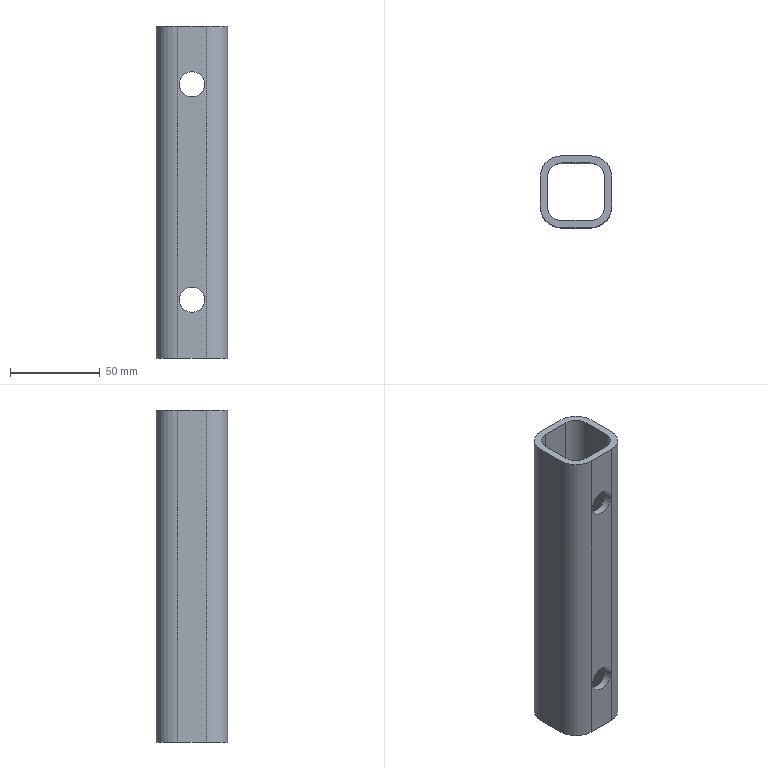Part | SolidWorks | features LayoutProfileFeature 1 | 1 solid | 26 faces | box 40 x 40 x 185 mm | volume 91393 mm3 | cylinder 16 | plane 10 | commonest cylinder face diameters 14 x8 16 x4 24 x4
STEP:
#1=CARTESIAN_POINT('',(7.,-20.,32.5));
#2=VERTEX_POINT('',#1);
#3=CARTESIAN_POINT('',(-7.,-20.,32.5));
#4=VERTEX_POINT('',#3);
#5=CARTESIAN_POINT('',(0.,-20.,32.5));
#6=DIRECTION('',(0.,1.,0.));
#7=DIRECTION('',(-1.,0.,0.));
#8=AXIS2_PLACEMENT_3D('',#5,#6,#7);
#9=CIRCLE('',#8,7.);
#10=EDGE_CURVE('',#2,#4,#9,.T.);
#11=ORIENTED_EDGE('',*,*,#10,.F.);
#12=CARTESIAN_POINT('',(7.,-16.,32.5));
#13=VERTEX_POINT('',#12);
#14=CARTESIAN_POINT('',(7.,-20.,32.5));
#15=DIRECTION('',(0.,1.,0.));
#16=VECTOR('',#15,1000.);
#17=LINE('',#14,#16);
#18=EDGE_CURVE('',#2,#13,#17,.T.);
#19=ORIENTED_EDGE('',*,*,#18,.T.);
#20=CARTESIAN_POINT('',(-7.,-16.,32.5));
#21=VERTEX_POINT('',#20);
#22=CARTESIAN_POINT('',(0.,-16.,32.5));
#23=DIRECTION('',(0.,1.,0.));
#24=DIRECTION('',(-1.,0.,0.));
#25=AXIS2_PLACEMENT_3D('',#22,#23,#24);
#26=CIRCLE('',#25,7.);
#27=EDGE_CURVE('',#13,#21,#26,.T.);
#28=ORIENTED_EDGE('',*,*,#27,.T.);
#29=CARTESIAN_POINT('',(-7.,-20.,32.5));
#30=DIRECTION('',(0.,1.,0.));
#31=VECTOR('',#30,1000.);
#32=LINE('',#29,#31);
#33=EDGE_CURVE('',#4,#21,#32,.T.);
#34=ORIENTED_EDGE('',*,*,#33,.F.);
#35=EDGE_LOOP('',(#11,#19,#28,#34));
#36=FACE_OUTER_BOUND('',#35,.T.);
#37=CARTESIAN_POINT('',(0.,-20.,32.5));
#38=DIRECTION('',(0.,1.,0.));
#39=DIRECTION('',(-1.,0.,0.));
#40=AXIS2_PLACEMENT_3D('',#37,#38,#39);
#41=CYLINDRICAL_SURFACE('',#40,7.);
#42=ADVANCED_FACE('',(#36),#41,.F.);
#43=CARTESIAN_POINT('',(7.,-20.,152.5));
#44=VERTEX_POINT('',#43);
#45=CARTESIAN_POINT('',(-7.,-20.,152.5));
#46=VERTEX_POINT('',#45);
#47=CARTESIAN_POINT('',(0.,-20.,152.5));
#48=DIRECTION('',(0.,1.,0.));
#49=DIRECTION('',(-1.,0.,0.));
#50=AXIS2_PLACEMENT_3D('',#47,#48,#49);
#51=CIRCLE('',#50,7.);
#52=EDGE_CURVE('',#44,#46,#51,.T.);
#53=ORIENTED_EDGE('',*,*,#52,.F.);
#54=CARTESIAN_POINT('',(7.,-16.,152.5));
#55=VERTEX_POINT('',#54);
#56=CARTESIAN_POINT('',(7.,-20.,152.5));
#57=DIRECTION('',(0.,1.,0.));
#58=VECTOR('',#57,1000.);
#59=LINE('',#56,#58);
#60=EDGE_CURVE('',#44,#55,#59,.T.);
#61=ORIENTED_EDGE('',*,*,#60,.T.);
#62=CARTESIAN_POINT('',(-7.,-16.,152.5));
#63=VERTEX_POINT('',#62);
#64=CARTESIAN_POINT('',(0.,-16.,152.5));
#65=DIRECTION('',(0.,1.,0.));
#66=DIRECTION('',(-1.,0.,0.));
#67=AXIS2_PLACEMENT_3D('',#64,#65,#66);
#68=CIRCLE('',#67,7.);
#69=EDGE_CURVE('',#55,#63,#68,.T.);
#70=ORIENTED_EDGE('',*,*,#69,.T.);
#71=CARTESIAN_POINT('',(-7.,-20.,152.5));
#72=DIRECTION('',(0.,1.,0.));
#73=VECTOR('',#72,1000.);
#74=LINE('',#71,#73);
#75=EDGE_CURVE('',#46,#63,#74,.T.);
#76=ORIENTED_EDGE('',*,*,#75,.F.);
#77=EDGE_LOOP('',(#53,#61,#70,#76));
#78=FACE_OUTER_BOUND('',#77,.T.);
#79=CARTESIAN_POINT('',(0.,-20.,152.5));
#80=DIRECTION('',(0.,1.,0.));
#81=DIRECTION('',(-1.,0.,0.));
#82=AXIS2_PLACEMENT_3D('',#79,#80,#81);
#83=CYLINDRICAL_SURFACE('',#82,7.);
#84=ADVANCED_FACE('',(#78),#83,.F.);
#85=CARTESIAN_POINT('',(-7.,16.,32.5));
#86=VERTEX_POINT('',#85);
#87=CARTESIAN_POINT('',(7.,16.,32.5));
#88=VERTEX_POINT('',#87);
#89=CARTESIAN_POINT('',(0.,16.,32.5));
#90=DIRECTION('',(0.,-1.,0.));
#91=DIRECTION('',(-1.,0.,0.));
#92=AXIS2_PLACEMENT_3D('',#89,#90,#91);
#93=CIRCLE('',#92,7.);
#94=EDGE_CURVE('',#86,#88,#93,.T.);
#95=ORIENTED_EDGE('',*,*,#94,.T.);
#96=CARTESIAN_POINT('',(7.,20.,32.5));
#97=VERTEX_POINT('',#96);
#98=CARTESIAN_POINT('',(7.,-20.,32.5));
#99=DIRECTION('',(0.,1.,0.));
#100=VECTOR('',#99,1000.);
#101=LINE('',#98,#100);
#102=EDGE_CURVE('',#88,#97,#101,.T.);
#103=ORIENTED_EDGE('',*,*,#102,.T.);
#104=CARTESIAN_POINT('',(-7.,20.,32.5));
#105=VERTEX_POINT('',#104);
#106=CARTESIAN_POINT('',(0.,20.,32.5));
#107=DIRECTION('',(0.,-1.,0.));
#108=DIRECTION('',(-1.,0.,0.));
#109=AXIS2_PLACEMENT_3D('',#106,#107,#108);
#110=CIRCLE('',#109,7.);
#111=EDGE_CURVE('',#105,#97,#110,.T.);
#112=ORIENTED_EDGE('',*,*,#111,.F.);
#113=CARTESIAN_POINT('',(-7.,-20.,32.5));
#114=DIRECTION('',(0.,1.,0.));
#115=VECTOR('',#114,1000.);
#116=LINE('',#113,#115);
#117=EDGE_CURVE('',#86,#105,#116,.T.);
#118=ORIENTED_EDGE('',*,*,#117,.F.);
#119=EDGE_LOOP('',(#95,#103,#112,#118));
#120=FACE_OUTER_BOUND('',#119,.T.);
#121=CARTESIAN_POINT('',(0.,-20.,32.5));
#122=DIRECTION('',(0.,1.,0.));
#123=DIRECTION('',(-1.,0.,0.));
#124=AXIS2_PLACEMENT_3D('',#121,#122,#123);
#125=CYLINDRICAL_SURFACE('',#124,7.);
#126=ADVANCED_FACE('',(#120),#125,.F.);
#127=CARTESIAN_POINT('',(-7.,16.,152.5));
#128=VERTEX_POINT('',#127);
#129=CARTESIAN_POINT('',(7.,16.,152.5));
#130=VERTEX_POINT('',#129);
#131=CARTESIAN_POINT('',(0.,16.,152.5));
#132=DIRECTION('',(0.,-1.,0.));
#133=DIRECTION('',(-1.,0.,0.));
#134=AXIS2_PLACEMENT_3D('',#131,#132,#133);
#135=CIRCLE('',#134,7.);
#136=EDGE_CURVE('',#128,#130,#135,.T.);
#137=ORIENTED_EDGE('',*,*,#136,.T.);
#138=CARTESIAN_POINT('',(7.,20.,152.5));
#139=VERTEX_POINT('',#138);
#140=CARTESIAN_POINT('',(7.,-20.,152.5));
#141=DIRECTION('',(0.,1.,0.));
#142=VECTOR('',#141,1000.);
#143=LINE('',#140,#142);
#144=EDGE_CURVE('',#130,#139,#143,.T.);
#145=ORIENTED_EDGE('',*,*,#144,.T.);
#146=CARTESIAN_POINT('',(-7.,20.,152.5));
#147=VERTEX_POINT('',#146);
#148=CARTESIAN_POINT('',(0.,20.,152.5));
#149=DIRECTION('',(0.,-1.,0.));
#150=DIRECTION('',(-1.,0.,0.));
#151=AXIS2_PLACEMENT_3D('',#148,#149,#150);
#152=CIRCLE('',#151,7.);
#153=EDGE_CURVE('',#147,#139,#152,.T.);
#154=ORIENTED_EDGE('',*,*,#153,.F.);
#155=CARTESIAN_POINT('',(-7.,-20.,152.5));
#156=DIRECTION('',(0.,1.,0.));
#157=VECTOR('',#156,1000.);
#158=LINE('',#155,#157);
#159=EDGE_CURVE('',#128,#147,#158,.T.);
#160=ORIENTED_EDGE('',*,*,#159,.F.);
#161=EDGE_LOOP('',(#137,#145,#154,#160));
#162=FACE_OUTER_BOUND('',#161,.T.);
#163=CARTESIAN_POINT('',(0.,-20.,152.5));
#164=DIRECTION('',(0.,1.,0.));
#165=DIRECTION('',(-1.,0.,0.));
#166=AXIS2_PLACEMENT_3D('',#163,#164,#165);
#167=CYLINDRICAL_SURFACE('',#166,7.);
#168=ADVANCED_FACE('',(#162),#167,.F.);
#169=CARTESIAN_POINT('',(8.,-20.,0.));
#170=VERTEX_POINT('',#169);
#171=CARTESIAN_POINT('',(20.,-8.,0.));
#172=VERTEX_POINT('',#171);
#173=CARTESIAN_POINT('',(8.,-8.,0.));
#174=DIRECTION('',(0.,0.,1.));
#175=DIRECTION('',(1.,0.,0.));
#176=AXIS2_PLACEMENT_3D('',#173,#174,#175);
#177=CIRCLE('',#176,12.);
#178=EDGE_CURVE('',#170,#172,#177,.T.);
#179=ORIENTED_EDGE('',*,*,#178,.T.);
#180=CARTESIAN_POINT('',(20.,-8.,185.));
#181=VERTEX_POINT('',#180);
#182=CARTESIAN_POINT('',(20.,-8.,0.));
#183=DIRECTION('',(0.,0.,1.));
#184=VECTOR('',#183,1000.);
#185=LINE('',#182,#184);
#186=EDGE_CURVE('',#172,#181,#185,.T.);
#187=ORIENTED_EDGE('',*,*,#186,.T.);
#188=CARTESIAN_POINT('',(8.,-20.,185.));
#189=VERTEX_POINT('',#188);
#190=CARTESIAN_POINT('',(8.,-8.,185.));
#191=DIRECTION('',(0.,0.,-1.));
#192=DIRECTION('',(1.,0.,0.));
#193=AXIS2_PLACEMENT_3D('',#190,#191,#192);
#194=CIRCLE('',#193,12.);
#195=EDGE_CURVE('',#181,#189,#194,.T.);
#196=ORIENTED_EDGE('',*,*,#195,.T.);
#197=CARTESIAN_POINT('',(8.,-20.,0.));
#198=DIRECTION('',(0.,0.,-1.));
#199=VECTOR('',#198,1000.);
#200=LINE('',#197,#199);
#201=EDGE_CURVE('',#189,#170,#200,.T.);
#202=ORIENTED_EDGE('',*,*,#201,.T.);
#203=EDGE_LOOP('',(#179,#187,#196,#202));
#204=FACE_OUTER_BOUND('',#203,.T.);
#205=CARTESIAN_POINT('',(8.,-8.,0.));
#206=DIRECTION('',(0.,0.,1.));
#207=DIRECTION('',(1.,0.,0.));
#208=AXIS2_PLACEMENT_3D('',#205,#206,#207);
#209=CYLINDRICAL_SURFACE('',#208,12.);
#210=ADVANCED_FACE('',(#204),#209,.T.);
#211=CARTESIAN_POINT('',(20.,8.,0.));
#212=VERTEX_POINT('',#211);
#213=CARTESIAN_POINT('',(20.,8.,0.));
#214=DIRECTION('',(0.,1.,0.));
#215=VECTOR('',#214,1000.);
#216=LINE('',#213,#215);
#217=EDGE_CURVE('',#172,#212,#216,.T.);
#218=ORIENTED_EDGE('',*,*,#217,.T.);
#219=CARTESIAN_POINT('',(20.,8.,185.));
#220=VERTEX_POINT('',#219);
#221=CARTESIAN_POINT('',(20.,8.,0.));
#222=DIRECTION('',(0.,0.,1.));
#223=VECTOR('',#222,1000.);
#224=LINE('',#221,#223);
#225=EDGE_CURVE('',#212,#220,#224,.T.);
#226=ORIENTED_EDGE('',*,*,#225,.T.);
#227=CARTESIAN_POINT('',(20.,8.,185.));
#228=DIRECTION('',(0.,-1.,0.));
#229=VECTOR('',#228,1000.);
#230=LINE('',#227,#229);
#231=EDGE_CURVE('',#220,#181,#230,.T.);
#232=ORIENTED_EDGE('',*,*,#231,.T.);
#233=ORIENTED_EDGE('',*,*,#186,.F.);
#234=EDGE_LOOP('',(#218,#226,#232,#233));
#235=FACE_OUTER_BOUND('',#234,.T.);
#236=CARTESIAN_POINT('',(20.,8.,0.));
#237=DIRECTION('',(1.,0.,0.));
#238=DIRECTION('',(0.,1.,0.));
#239=AXIS2_PLACEMENT_3D('',#236,#237,#238);
#240=PLANE('',#239);
#241=ADVANCED_FACE('',(#235),#240,.T.);
#242=CARTESIAN_POINT('',(-16.,8.,0.));
#243=VERTEX_POINT('',#242);
#244=CARTESIAN_POINT('',(-8.,16.,0.));
#245=VERTEX_POINT('',#244);
#246=CARTESIAN_POINT('',(-8.,8.,0.));
#247=DIRECTION('',(0.,0.,-1.));
#248=DIRECTION('',(1.,0.,0.));
#249=AXIS2_PLACEMENT_3D('',#246,#247,#248);
#250=CIRCLE('',#249,8.);
#251=EDGE_CURVE('',#243,#245,#250,.T.);
#252=ORIENTED_EDGE('',*,*,#251,.F.);
#253=CARTESIAN_POINT('',(-16.,-8.,0.));
#254=VERTEX_POINT('',#253);
#255=CARTESIAN_POINT('',(-16.,0.,0.));
#256=DIRECTION('',(0.,1.,0.));
#257=VECTOR('',#256,1000.);
#258=LINE('',#255,#257);
#259=EDGE_CURVE('',#254,#243,#258,.T.);
#260=ORIENTED_EDGE('',*,*,#259,.F.);
#261=CARTESIAN_POINT('',(-8.,-16.,0.));
#262=VERTEX_POINT('',#261);
#263=CARTESIAN_POINT('',(-8.,-8.,0.));
#264=DIRECTION('',(0.,0.,-1.));
#265=DIRECTION('',(1.,0.,0.));
#266=AXIS2_PLACEMENT_3D('',#263,#264,#265);
#267=CIRCLE('',#266,8.);
#268=EDGE_CURVE('',#262,#254,#267,.T.);
#269=ORIENTED_EDGE('',*,*,#268,.F.);
#270=CARTESIAN_POINT('',(8.,-16.,0.));
#271=VERTEX_POINT('',#270);
#272=CARTESIAN_POINT('',(0.,-16.,0.));
#273=DIRECTION('',(-1.,0.,0.));
#274=VECTOR('',#273,1000.);
#275=LINE('',#272,#274);
#276=EDGE_CURVE('',#271,#262,#275,.T.);
#277=ORIENTED_EDGE('',*,*,#276,.F.);
#278=CARTESIAN_POINT('',(16.,-8.,0.));
#279=VERTEX_POINT('',#278);
#280=CARTESIAN_POINT('',(8.,-8.,0.));
#281=DIRECTION('',(0.,0.,-1.));
#282=DIRECTION('',(1.,0.,0.));
#283=AXIS2_PLACEMENT_3D('',#280,#281,#282);
#284=CIRCLE('',#283,8.);
#285=EDGE_CURVE('',#279,#271,#284,.T.);
#286=ORIENTED_EDGE('',*,*,#285,.F.);
#287=CARTESIAN_POINT('',(16.,8.,0.));
#288=VERTEX_POINT('',#287);
#289=CARTESIAN_POINT('',(16.,0.,0.));
#290=DIRECTION('',(0.,-1.,0.));
#291=VECTOR('',#290,1000.);
#292=LINE('',#289,#291);
#293=EDGE_CURVE('',#288,#279,#292,.T.);
#294=ORIENTED_EDGE('',*,*,#293,.F.);
#295=CARTESIAN_POINT('',(8.,16.,0.));
#296=VERTEX_POINT('',#295);
#297=CARTESIAN_POINT('',(8.,8.,0.));
#298=DIRECTION('',(0.,0.,-1.));
#299=DIRECTION('',(1.,0.,0.));
#300=AXIS2_PLACEMENT_3D('',#297,#298,#299);
#301=CIRCLE('',#300,8.);
#302=EDGE_CURVE('',#296,#288,#301,.T.);
#303=ORIENTED_EDGE('',*,*,#302,.F.);
#304=CARTESIAN_POINT('',(0.,16.,0.));
#305=DIRECTION('',(1.,0.,0.));
#306=VECTOR('',#305,1000.);
#307=LINE('',#304,#306);
#308=EDGE_CURVE('',#245,#296,#307,.T.);
#309=ORIENTED_EDGE('',*,*,#308,.F.);
#310=EDGE_LOOP('',(#252,#260,#269,#277,#286,#294,#303,#309));
#311=FACE_BOUND('',#310,.T.);
#312=CARTESIAN_POINT('',(-8.,20.,0.));
#313=VERTEX_POINT('',#312);
#314=CARTESIAN_POINT('',(-20.,8.,0.));
#315=VERTEX_POINT('',#314);
#316=CARTESIAN_POINT('',(-8.,8.,0.));
#317=DIRECTION('',(0.,0.,1.));
#318=DIRECTION('',(1.,0.,0.));
#319=AXIS2_PLACEMENT_3D('',#316,#317,#318);
#320=CIRCLE('',#319,12.);
#321=EDGE_CURVE('',#313,#315,#320,.T.);
#322=ORIENTED_EDGE('',*,*,#321,.F.);
#323=CARTESIAN_POINT('',(8.,20.,0.));
#324=VERTEX_POINT('',#323);
#325=CARTESIAN_POINT('',(0.,20.,0.));
#326=DIRECTION('',(-1.,0.,0.));
#327=VECTOR('',#326,1000.);
#328=LINE('',#325,#327);
#329=EDGE_CURVE('',#324,#313,#328,.T.);
#330=ORIENTED_EDGE('',*,*,#329,.F.);
#331=CARTESIAN_POINT('',(8.,8.,0.));
#332=DIRECTION('',(0.,0.,1.));
#333=DIRECTION('',(1.,0.,0.));
#334=AXIS2_PLACEMENT_3D('',#331,#332,#333);
#335=CIRCLE('',#334,12.);
#336=EDGE_CURVE('',#212,#324,#335,.T.);
#337=ORIENTED_EDGE('',*,*,#336,.F.);
#338=ORIENTED_EDGE('',*,*,#217,.F.);
#339=ORIENTED_EDGE('',*,*,#178,.F.);
#340=CARTESIAN_POINT('',(-8.,-20.,0.));
#341=VERTEX_POINT('',#340);
#342=CARTESIAN_POINT('',(0.,-20.,0.));
#343=DIRECTION('',(1.,0.,0.));
#344=VECTOR('',#343,1000.);
#345=LINE('',#342,#344);
#346=EDGE_CURVE('',#341,#170,#345,.T.);
#347=ORIENTED_EDGE('',*,*,#346,.F.);
#348=CARTESIAN_POINT('',(-20.,-8.,0.));
#349=VERTEX_POINT('',#348);
#350=CARTESIAN_POINT('',(-8.,-8.,0.));
#351=DIRECTION('',(0.,0.,1.));
#352=DIRECTION('',(1.,0.,0.));
#353=AXIS2_PLACEMENT_3D('',#350,#351,#352);
#354=CIRCLE('',#353,12.);
#355=EDGE_CURVE('',#349,#341,#354,.T.);
#356=ORIENTED_EDGE('',*,*,#355,.F.);
#357=CARTESIAN_POINT('',(-20.,0.,0.));
#358=DIRECTION('',(0.,-1.,0.));
#359=VECTOR('',#358,1000.);
#360=LINE('',#357,#359);
#361=EDGE_CURVE('',#315,#349,#360,.T.);
#362=ORIENTED_EDGE('',*,*,#361,.F.);
#363=EDGE_LOOP('',(#322,#330,#337,#338,#339,#347,#356,#362));
#364=FACE_OUTER_BOUND('',#363,.T.);
#365=CARTESIAN_POINT('',(0.,0.,0.));
#366=DIRECTION('',(0.,0.,1.));
#367=DIRECTION('',(1.,0.,0.));
#368=AXIS2_PLACEMENT_3D('',#365,#366,#367);
#369=PLANE('',#368);
#370=ADVANCED_FACE('',(#311,#364),#369,.F.);
#371=CARTESIAN_POINT('',(0.,-20.,32.5));
#372=DIRECTION('',(0.,1.,0.));
#373=DIRECTION('',(-1.,0.,0.));
#374=AXIS2_PLACEMENT_3D('',#371,#372,#373);
#375=CIRCLE('',#374,7.);
#376=EDGE_CURVE('',#4,#2,#375,.T.);
#377=ORIENTED_EDGE('',*,*,#376,.T.);
#378=ORIENTED_EDGE('',*,*,#10,.T.);
#379=EDGE_LOOP('',(#377,#378));
#380=FACE_BOUND('',#379,.T.);
#381=CARTESIAN_POINT('',(0.,-20.,152.5));
#382=DIRECTION('',(0.,1.,0.));
#383=DIRECTION('',(-1.,0.,0.));
#384=AXIS2_PLACEMENT_3D('',#381,#382,#383);
#385=CIRCLE('',#384,7.);
#386=EDGE_CURVE('',#46,#44,#385,.T.);
#387=ORIENTED_EDGE('',*,*,#386,.T.);
#388=ORIENTED_EDGE('',*,*,#52,.T.);
#389=EDGE_LOOP('',(#387,#388));
#390=FACE_BOUND('',#389,.T.);
#391=ORIENTED_EDGE('',*,*,#346,.T.);
#392=ORIENTED_EDGE('',*,*,#201,.F.);
#393=CARTESIAN_POINT('',(-8.,-20.,185.));
#394=VERTEX_POINT('',#393);
#395=CARTESIAN_POINT('',(8.,-20.,185.));
#396=DIRECTION('',(-1.,0.,0.));
#397=VECTOR('',#396,1000.);
#398=LINE('',#395,#397);
#399=EDGE_CURVE('',#189,#394,#398,.T.);
#400=ORIENTED_EDGE('',*,*,#399,.T.);
#401=CARTESIAN_POINT('',(-8.,-20.,0.));
#402=DIRECTION('',(0.,0.,-1.));
#403=VECTOR('',#402,1000.);
#404=LINE('',#401,#403);
#405=EDGE_CURVE('',#394,#341,#404,.T.);
#406=ORIENTED_EDGE('',*,*,#405,.T.);
#407=EDGE_LOOP('',(#391,#392,#400,#406));
#408=FACE_OUTER_BOUND('',#407,.T.);
#409=CARTESIAN_POINT('',(8.,-20.,0.));
#410=DIRECTION('',(0.,-1.,0.));
#411=DIRECTION('',(1.,0.,0.));
#412=AXIS2_PLACEMENT_3D('',#409,#410,#411);
#413=PLANE('',#412);
#414=ADVANCED_FACE('',(#380,#390,#408),#413,.T.);
#415=CARTESIAN_POINT('',(-16.,-8.,185.));
#416=VERTEX_POINT('',#415);
#417=CARTESIAN_POINT('',(-16.,8.,185.));
#418=VERTEX_POINT('',#417);
#419=CARTESIAN_POINT('',(-16.,0.,185.));
#420=DIRECTION('',(0.,1.,0.));
#421=VECTOR('',#420,1000.);
#422=LINE('',#419,#421);
#423=EDGE_CURVE('',#416,#418,#422,.T.);
#424=ORIENTED_EDGE('',*,*,#423,.T.);
#425=CARTESIAN_POINT('',(-8.,16.,185.));
#426=VERTEX_POINT('',#425);
#427=CARTESIAN_POINT('',(-8.,8.,185.));
#428=DIRECTION('',(0.,0.,-1.));
#429=DIRECTION('',(1.,0.,0.));
#430=AXIS2_PLACEMENT_3D('',#427,#428,#429);
#431=CIRCLE('',#430,8.);
#432=EDGE_CURVE('',#418,#426,#431,.T.);
#433=ORIENTED_EDGE('',*,*,#432,.T.);
#434=CARTESIAN_POINT('',(8.,16.,185.));
#435=VERTEX_POINT('',#434);
#436=CARTESIAN_POINT('',(0.,16.,185.));
#437=DIRECTION('',(1.,0.,0.));
#438=VECTOR('',#437,1000.);
#439=LINE('',#436,#438);
#440=EDGE_CURVE('',#426,#435,#439,.T.);
#441=ORIENTED_EDGE('',*,*,#440,.T.);
#442=CARTESIAN_POINT('',(16.,8.,185.));
#443=VERTEX_POINT('',#442);
#444=CARTESIAN_POINT('',(8.,8.,185.));
#445=DIRECTION('',(0.,0.,-1.));
#446=DIRECTION('',(1.,0.,0.));
#447=AXIS2_PLACEMENT_3D('',#444,#445,#446);
#448=CIRCLE('',#447,8.);
#449=EDGE_CURVE('',#435,#443,#448,.T.);
#450=ORIENTED_EDGE('',*,*,#449,.T.);
#451=CARTESIAN_POINT('',(16.,-8.,185.));
#452=VERTEX_POINT('',#451);
#453=CARTESIAN_POINT('',(16.,0.,185.));
#454=DIRECTION('',(0.,-1.,0.));
#455=VECTOR('',#454,1000.);
#456=LINE('',#453,#455);
#457=EDGE_CURVE('',#443,#452,#456,.T.);
#458=ORIENTED_EDGE('',*,*,#457,.T.);
#459=CARTESIAN_POINT('',(8.,-16.,185.));
#460=VERTEX_POINT('',#459);
#461=CARTESIAN_POINT('',(8.,-8.,185.));
#462=DIRECTION('',(0.,0.,-1.));
#463=DIRECTION('',(1.,0.,0.));
#464=AXIS2_PLACEMENT_3D('',#461,#462,#463);
#465=CIRCLE('',#464,8.);
#466=EDGE_CURVE('',#452,#460,#465,.T.);
#467=ORIENTED_EDGE('',*,*,#466,.T.);
#468=CARTESIAN_POINT('',(-8.,-16.,185.));
#469=VERTEX_POINT('',#468);
#470=CARTESIAN_POINT('',(0.,-16.,185.));
#471=DIRECTION('',(-1.,0.,0.));
#472=VECTOR('',#471,1000.);
#473=LINE('',#470,#472);
#474=EDGE_CURVE('',#460,#469,#473,.T.);
#475=ORIENTED_EDGE('',*,*,#474,.T.);
#476=CARTESIAN_POINT('',(-8.,-8.,185.));
#477=DIRECTION('',(0.,0.,-1.));
#478=DIRECTION('',(1.,0.,0.));
#479=AXIS2_PLACEMENT_3D('',#476,#477,#478);
#480=CIRCLE('',#479,8.);
#481=EDGE_CURVE('',#469,#416,#480,.T.);
#482=ORIENTED_EDGE('',*,*,#481,.T.);
#483=EDGE_LOOP('',(#424,#433,#441,#450,#458,#467,#475,#482));
#484=FACE_BOUND('',#483,.T.);
#485=CARTESIAN_POINT('',(8.,20.,185.));
#486=VERTEX_POINT('',#485);
#487=CARTESIAN_POINT('',(-8.,20.,185.));
#488=VERTEX_POINT('',#487);
#489=CARTESIAN_POINT('',(0.,20.,185.));
#490=DIRECTION('',(-1.,0.,0.));
#491=VECTOR('',#490,1000.);
#492=LINE('',#489,#491);
#493=EDGE_CURVE('',#486,#488,#492,.T.);
#494=ORIENTED_EDGE('',*,*,#493,.T.);
#495=CARTESIAN_POINT('',(-20.,8.,185.));
#496=VERTEX_POINT('',#495);
#497=CARTESIAN_POINT('',(-8.,8.,185.));
#498=DIRECTION('',(0.,0.,1.));
#499=DIRECTION('',(1.,0.,0.));
#500=AXIS2_PLACEMENT_3D('',#497,#498,#499);
#501=CIRCLE('',#500,12.);
#502=EDGE_CURVE('',#488,#496,#501,.T.);
#503=ORIENTED_EDGE('',*,*,#502,.T.);
#504=CARTESIAN_POINT('',(-20.,-8.,185.));
#505=VERTEX_POINT('',#504);
#506=CARTESIAN_POINT('',(-20.,0.,185.));
#507=DIRECTION('',(0.,-1.,0.));
#508=VECTOR('',#507,1000.);
#509=LINE('',#506,#508);
#510=EDGE_CURVE('',#496,#505,#509,.T.);
#511=ORIENTED_EDGE('',*,*,#510,.T.);
#512=CARTESIAN_POINT('',(-8.,-8.,185.));
#513=DIRECTION('',(0.,0.,1.));
#514=DIRECTION('',(1.,0.,0.));
#515=AXIS2_PLACEMENT_3D('',#512,#513,#514);
#516=CIRCLE('',#515,12.);
#517=EDGE_CURVE('',#505,#394,#516,.T.);
#518=ORIENTED_EDGE('',*,*,#517,.T.);
#519=ORIENTED_EDGE('',*,*,#399,.F.);
#520=ORIENTED_EDGE('',*,*,#195,.F.);
#521=ORIENTED_EDGE('',*,*,#231,.F.);
#522=CARTESIAN_POINT('',(8.,8.,185.));
#523=DIRECTION('',(0.,0.,1.));
#524=DIRECTION('',(1.,0.,0.));
#525=AXIS2_PLACEMENT_3D('',#522,#523,#524);
#526=CIRCLE('',#525,12.);
#527=EDGE_CURVE('',#220,#486,#526,.T.);
#528=ORIENTED_EDGE('',*,*,#527,.T.);
#529=EDGE_LOOP('',(#494,#503,#511,#518,#519,#520,#521,#528));
#530=FACE_OUTER_BOUND('',#529,.T.);
#531=CARTESIAN_POINT('',(0.,0.,185.));
#532=DIRECTION('',(0.,0.,1.));
#533=DIRECTION('',(1.,0.,0.));
#534=AXIS2_PLACEMENT_3D('',#531,#532,#533);
#535=PLANE('',#534);
#536=ADVANCED_FACE('',(#484,#530),#535,.T.);
#537=ORIENTED_EDGE('',*,*,#336,.T.);
#538=CARTESIAN_POINT('',(8.,20.,0.));
#539=DIRECTION('',(0.,0.,1.));
#540=VECTOR('',#539,1000.);
#541=LINE('',#538,#540);
#542=EDGE_CURVE('',#324,#486,#541,.T.);
#543=ORIENTED_EDGE('',*,*,#542,.T.);
#544=ORIENTED_EDGE('',*,*,#527,.F.);
#545=ORIENTED_EDGE('',*,*,#225,.F.);
#546=EDGE_LOOP('',(#537,#543,#544,#545));
#547=FACE_OUTER_BOUND('',#546,.T.);
#548=CARTESIAN_POINT('',(8.,8.,0.));
#549=DIRECTION('',(0.,0.,1.));
#550=DIRECTION('',(1.,0.,0.));
#551=AXIS2_PLACEMENT_3D('',#548,#549,#550);
#552=CYLINDRICAL_SURFACE('',#551,12.);
#553=ADVANCED_FACE('',(#547),#552,.T.);
#554=ORIENTED_EDGE('',*,*,#94,.F.);
#555=CARTESIAN_POINT('',(0.,16.,32.5));
#556=DIRECTION('',(0.,-1.,0.));
#557=DIRECTION('',(-1.,0.,0.));
#558=AXIS2_PLACEMENT_3D('',#555,#556,#557);
#559=CIRCLE('',#558,7.);
#560=EDGE_CURVE('',#88,#86,#559,.T.);
#561=ORIENTED_EDGE('',*,*,#560,.F.);
#562=EDGE_LOOP('',(#554,#561));
#563=FACE_BOUND('',#562,.T.);
#564=ORIENTED_EDGE('',*,*,#136,.F.);
#565=CARTESIAN_POINT('',(0.,16.,152.5));
#566=DIRECTION('',(0.,-1.,0.));
#567=DIRECTION('',(-1.,0.,0.));
#568=AXIS2_PLACEMENT_3D('',#565,#566,#567);
#569=CIRCLE('',#568,7.);
#570=EDGE_CURVE('',#130,#128,#569,.T.);
#571=ORIENTED_EDGE('',*,*,#570,.F.);
#572=EDGE_LOOP('',(#564,#571));
#573=FACE_BOUND('',#572,.T.);
#574=CARTESIAN_POINT('',(-8.,16.,0.));
#575=DIRECTION('',(0.,0.,1.));
#576=VECTOR('',#575,1000.);
#577=LINE('',#574,#576);
#578=EDGE_CURVE('',#245,#426,#577,.T.);
#579=ORIENTED_EDGE('',*,*,#578,.F.);
#580=ORIENTED_EDGE('',*,*,#308,.T.);
#581=CARTESIAN_POINT('',(8.,16.,0.));
#582=DIRECTION('',(0.,0.,-1.));
#583=VECTOR('',#582,1000.);
#584=LINE('',#581,#583);
#585=EDGE_CURVE('',#435,#296,#584,.T.);
#586=ORIENTED_EDGE('',*,*,#585,.F.);
#587=ORIENTED_EDGE('',*,*,#440,.F.);
#588=EDGE_LOOP('',(#579,#580,#586,#587));
#589=FACE_OUTER_BOUND('',#588,.T.);
#590=CARTESIAN_POINT('',(-8.,16.,0.));
#591=DIRECTION('',(0.,1.,0.));
#592=DIRECTION('',(-1.,0.,0.));
#593=AXIS2_PLACEMENT_3D('',#590,#591,#592);
#594=PLANE('',#593);
#595=ADVANCED_FACE('',(#563,#573,#589),#594,.F.);
#596=CARTESIAN_POINT('',(-16.,8.,0.));
#597=DIRECTION('',(0.,0.,1.));
#598=VECTOR('',#597,1000.);
#599=LINE('',#596,#598);
#600=EDGE_CURVE('',#243,#418,#599,.T.);
#601=ORIENTED_EDGE('',*,*,#600,.F.);
#602=ORIENTED_EDGE('',*,*,#251,.T.);
#603=ORIENTED_EDGE('',*,*,#578,.T.);
#604=ORIENTED_EDGE('',*,*,#432,.F.);
#605=EDGE_LOOP('',(#601,#602,#603,#604));
#606=FACE_OUTER_BOUND('',#605,.T.);
#607=CARTESIAN_POINT('',(-8.,8.,0.));
#608=DIRECTION('',(0.,0.,1.));
#609=DIRECTION('',(1.,0.,0.));
#610=AXIS2_PLACEMENT_3D('',#607,#608,#609);
#611=CYLINDRICAL_SURFACE('',#610,8.);
#612=ADVANCED_FACE('',(#606),#611,.F.);
#613=CARTESIAN_POINT('',(-16.,-8.,0.));
#614=DIRECTION('',(0.,0.,1.));
#615=VECTOR('',#614,1000.);
#616=LINE('',#613,#615);
#617=EDGE_CURVE('',#254,#416,#616,.T.);
#618=ORIENTED_EDGE('',*,*,#617,.F.);
#619=ORIENTED_EDGE('',*,*,#259,.T.);
#620=ORIENTED_EDGE('',*,*,#600,.T.);
#621=ORIENTED_EDGE('',*,*,#423,.F.);
#622=EDGE_LOOP('',(#618,#619,#620,#621));
#623=FACE_OUTER_BOUND('',#622,.T.);
#624=CARTESIAN_POINT('',(-16.,-8.,0.));
#625=DIRECTION('',(-1.,0.,0.));
#626=DIRECTION('',(0.,-1.,0.));
#627=AXIS2_PLACEMENT_3D('',#624,#625,#626);
#628=PLANE('',#627);
#629=ADVANCED_FACE('',(#623),#628,.F.);
#630=CARTESIAN_POINT('',(-8.,-16.,0.));
#631=DIRECTION('',(0.,0.,1.));
#632=VECTOR('',#631,1000.);
#633=LINE('',#630,#632);
#634=EDGE_CURVE('',#262,#469,#633,.T.);
#635=ORIENTED_EDGE('',*,*,#634,.F.);
#636=ORIENTED_EDGE('',*,*,#268,.T.);
#637=ORIENTED_EDGE('',*,*,#617,.T.);
#638=ORIENTED_EDGE('',*,*,#481,.F.);
#639=EDGE_LOOP('',(#635,#636,#637,#638));
#640=FACE_OUTER_BOUND('',#639,.T.);
#641=CARTESIAN_POINT('',(-8.,-8.,0.));
#642=DIRECTION('',(0.,0.,1.));
#643=DIRECTION('',(1.,0.,0.));
#644=AXIS2_PLACEMENT_3D('',#641,#642,#643);
#645=CYLINDRICAL_SURFACE('',#644,8.);
#646=ADVANCED_FACE('',(#640),#645,.F.);
#647=CARTESIAN_POINT('',(0.,-16.,32.5));
#648=DIRECTION('',(0.,1.,0.));
#649=DIRECTION('',(-1.,0.,0.));
#650=AXIS2_PLACEMENT_3D('',#647,#648,#649);
#651=CIRCLE('',#650,7.);
#652=EDGE_CURVE('',#21,#13,#651,.T.);
#653=ORIENTED_EDGE('',*,*,#652,.F.);
#654=ORIENTED_EDGE('',*,*,#27,.F.);
#655=EDGE_LOOP('',(#653,#654));
#656=FACE_BOUND('',#655,.T.);
#657=CARTESIAN_POINT('',(0.,-16.,152.5));
#658=DIRECTION('',(0.,1.,0.));
#659=DIRECTION('',(-1.,0.,0.));
#660=AXIS2_PLACEMENT_3D('',#657,#658,#659);
#661=CIRCLE('',#660,7.);
#662=EDGE_CURVE('',#63,#55,#661,.T.);
#663=ORIENTED_EDGE('',*,*,#662,.F.);
#664=ORIENTED_EDGE('',*,*,#69,.F.);
#665=EDGE_LOOP('',(#663,#664));
#666=FACE_BOUND('',#665,.T.);
#667=CARTESIAN_POINT('',(8.,-16.,0.));
#668=DIRECTION('',(0.,0.,1.));
#669=VECTOR('',#668,1000.);
#670=LINE('',#667,#669);
#671=EDGE_CURVE('',#271,#460,#670,.T.);
#672=ORIENTED_EDGE('',*,*,#671,.F.);
#673=ORIENTED_EDGE('',*,*,#276,.T.);
#674=ORIENTED_EDGE('',*,*,#634,.T.);
#675=ORIENTED_EDGE('',*,*,#474,.F.);
#676=EDGE_LOOP('',(#672,#673,#674,#675));
#677=FACE_OUTER_BOUND('',#676,.T.);
#678=CARTESIAN_POINT('',(8.,-16.,0.));
#679=DIRECTION('',(0.,-1.,0.));
#680=DIRECTION('',(1.,0.,0.));
#681=AXIS2_PLACEMENT_3D('',#678,#679,#680);
#682=PLANE('',#681);
#683=ADVANCED_FACE('',(#656,#666,#677),#682,.F.);
#684=CARTESIAN_POINT('',(16.,-8.,0.));
#685=DIRECTION('',(0.,0.,1.));
#686=VECTOR('',#685,1000.);
#687=LINE('',#684,#686);
#688=EDGE_CURVE('',#279,#452,#687,.T.);
#689=ORIENTED_EDGE('',*,*,#688,.F.);
#690=ORIENTED_EDGE('',*,*,#285,.T.);
#691=ORIENTED_EDGE('',*,*,#671,.T.);
#692=ORIENTED_EDGE('',*,*,#466,.F.);
#693=EDGE_LOOP('',(#689,#690,#691,#692));
#694=FACE_OUTER_BOUND('',#693,.T.);
#695=CARTESIAN_POINT('',(8.,-8.,0.));
#696=DIRECTION('',(0.,0.,1.));
#697=DIRECTION('',(1.,0.,0.));
#698=AXIS2_PLACEMENT_3D('',#695,#696,#697);
#699=CYLINDRICAL_SURFACE('',#698,8.);
#700=ADVANCED_FACE('',(#694),#699,.F.);
#701=CARTESIAN_POINT('',(16.,8.,0.));
#702=DIRECTION('',(0.,0.,1.));
#703=VECTOR('',#702,1000.);
#704=LINE('',#701,#703);
#705=EDGE_CURVE('',#288,#443,#704,.T.);
#706=ORIENTED_EDGE('',*,*,#705,.F.);
#707=ORIENTED_EDGE('',*,*,#293,.T.);
#708=ORIENTED_EDGE('',*,*,#688,.T.);
#709=ORIENTED_EDGE('',*,*,#457,.F.);
#710=EDGE_LOOP('',(#706,#707,#708,#709));
#711=FACE_OUTER_BOUND('',#710,.T.);
#712=CARTESIAN_POINT('',(16.,8.,0.));
#713=DIRECTION('',(1.,0.,0.));
#714=DIRECTION('',(0.,0.,-1.));
#715=AXIS2_PLACEMENT_3D('',#712,#713,#714);
#716=PLANE('',#715);
#717=ADVANCED_FACE('',(#711),#716,.F.);
#718=ORIENTED_EDGE('',*,*,#585,.T.);
#719=ORIENTED_EDGE('',*,*,#302,.T.);
#720=ORIENTED_EDGE('',*,*,#705,.T.);
#721=ORIENTED_EDGE('',*,*,#449,.F.);
#722=EDGE_LOOP('',(#718,#719,#720,#721));
#723=FACE_OUTER_BOUND('',#722,.T.);
#724=CARTESIAN_POINT('',(8.,8.,0.));
#725=DIRECTION('',(0.,0.,1.));
#726=DIRECTION('',(1.,0.,0.));
#727=AXIS2_PLACEMENT_3D('',#724,#725,#726);
#728=CYLINDRICAL_SURFACE('',#727,8.);
#729=ADVANCED_FACE('',(#723),#728,.F.);
#730=ORIENTED_EDGE('',*,*,#361,.T.);
#731=CARTESIAN_POINT('',(-20.,-8.,0.));
#732=DIRECTION('',(0.,0.,1.));
#733=VECTOR('',#732,1000.);
#734=LINE('',#731,#733);
#735=EDGE_CURVE('',#349,#505,#734,.T.);
#736=ORIENTED_EDGE('',*,*,#735,.T.);
#737=ORIENTED_EDGE('',*,*,#510,.F.);
#738=CARTESIAN_POINT('',(-20.,8.,0.));
#739=DIRECTION('',(0.,0.,-1.));
#740=VECTOR('',#739,1000.);
#741=LINE('',#738,#740);
#742=EDGE_CURVE('',#496,#315,#741,.T.);
#743=ORIENTED_EDGE('',*,*,#742,.T.);
#744=EDGE_LOOP('',(#730,#736,#737,#743));
#745=FACE_OUTER_BOUND('',#744,.T.);
#746=CARTESIAN_POINT('',(-20.,-8.,0.));
#747=DIRECTION('',(-1.,0.,0.));
#748=DIRECTION('',(0.,-1.,0.));
#749=AXIS2_PLACEMENT_3D('',#746,#747,#748);
#750=PLANE('',#749);
#751=ADVANCED_FACE('',(#745),#750,.T.);
#752=ORIENTED_EDGE('',*,*,#321,.T.);
#753=ORIENTED_EDGE('',*,*,#742,.F.);
#754=ORIENTED_EDGE('',*,*,#502,.F.);
#755=CARTESIAN_POINT('',(-8.,20.,0.));
#756=DIRECTION('',(0.,0.,-1.));
#757=VECTOR('',#756,1000.);
#758=LINE('',#755,#757);
#759=EDGE_CURVE('',#488,#313,#758,.T.);
#760=ORIENTED_EDGE('',*,*,#759,.T.);
#761=EDGE_LOOP('',(#752,#753,#754,#760));
#762=FACE_OUTER_BOUND('',#761,.T.);
#763=CARTESIAN_POINT('',(-8.,8.,0.));
#764=DIRECTION('',(0.,0.,1.));
#765=DIRECTION('',(1.,0.,0.));
#766=AXIS2_PLACEMENT_3D('',#763,#764,#765);
#767=CYLINDRICAL_SURFACE('',#766,12.);
#768=ADVANCED_FACE('',(#762),#767,.T.);
#769=ORIENTED_EDGE('',*,*,#111,.T.);
#770=CARTESIAN_POINT('',(0.,20.,32.5));
#771=DIRECTION('',(0.,-1.,0.));
#772=DIRECTION('',(-1.,0.,0.));
#773=AXIS2_PLACEMENT_3D('',#770,#771,#772);
#774=CIRCLE('',#773,7.);
#775=EDGE_CURVE('',#97,#105,#774,.T.);
#776=ORIENTED_EDGE('',*,*,#775,.T.);
#777=EDGE_LOOP('',(#769,#776));
#778=FACE_BOUND('',#777,.T.);
#779=ORIENTED_EDGE('',*,*,#153,.T.);
#780=CARTESIAN_POINT('',(0.,20.,152.5));
#781=DIRECTION('',(0.,-1.,0.));
#782=DIRECTION('',(-1.,0.,0.));
#783=AXIS2_PLACEMENT_3D('',#780,#781,#782);
#784=CIRCLE('',#783,7.);
#785=EDGE_CURVE('',#139,#147,#784,.T.);
#786=ORIENTED_EDGE('',*,*,#785,.T.);
#787=EDGE_LOOP('',(#779,#786));
#788=FACE_BOUND('',#787,.T.);
#789=ORIENTED_EDGE('',*,*,#329,.T.);
#790=ORIENTED_EDGE('',*,*,#759,.F.);
#791=ORIENTED_EDGE('',*,*,#493,.F.);
#792=ORIENTED_EDGE('',*,*,#542,.F.);
#793=EDGE_LOOP('',(#789,#790,#791,#792));
#794=FACE_OUTER_BOUND('',#793,.T.);
#795=CARTESIAN_POINT('',(-8.,20.,0.));
#796=DIRECTION('',(0.,1.,0.));
#797=DIRECTION('',(0.,0.,1.));
#798=AXIS2_PLACEMENT_3D('',#795,#796,#797);
#799=PLANE('',#798);
#800=ADVANCED_FACE('',(#778,#788,#794),#799,.T.);
#801=ORIENTED_EDGE('',*,*,#355,.T.);
#802=ORIENTED_EDGE('',*,*,#405,.F.);
#803=ORIENTED_EDGE('',*,*,#517,.F.);
#804=ORIENTED_EDGE('',*,*,#735,.F.);
#805=EDGE_LOOP('',(#801,#802,#803,#804));
#806=FACE_OUTER_BOUND('',#805,.T.);
#807=CARTESIAN_POINT('',(-8.,-8.,0.));
#808=DIRECTION('',(0.,0.,1.));
#809=DIRECTION('',(1.,0.,0.));
#810=AXIS2_PLACEMENT_3D('',#807,#808,#809);
#811=CYLINDRICAL_SURFACE('',#810,12.);
#812=ADVANCED_FACE('',(#806),#811,.T.);
#813=ORIENTED_EDGE('',*,*,#18,.F.);
#814=ORIENTED_EDGE('',*,*,#376,.F.);
#815=ORIENTED_EDGE('',*,*,#33,.T.);
#816=ORIENTED_EDGE('',*,*,#652,.T.);
#817=EDGE_LOOP('',(#813,#814,#815,#816));
#818=FACE_OUTER_BOUND('',#817,.T.);
#819=CARTESIAN_POINT('',(0.,-20.,32.5));
#820=DIRECTION('',(0.,1.,0.));
#821=DIRECTION('',(-1.,0.,0.));
#822=AXIS2_PLACEMENT_3D('',#819,#820,#821);
#823=CYLINDRICAL_SURFACE('',#822,7.);
#824=ADVANCED_FACE('',(#818),#823,.F.);
#825=ORIENTED_EDGE('',*,*,#60,.F.);
#826=ORIENTED_EDGE('',*,*,#386,.F.);
#827=ORIENTED_EDGE('',*,*,#75,.T.);
#828=ORIENTED_EDGE('',*,*,#662,.T.);
#829=EDGE_LOOP('',(#825,#826,#827,#828));
#830=FACE_OUTER_BOUND('',#829,.T.);
#831=CARTESIAN_POINT('',(0.,-20.,152.5));
#832=DIRECTION('',(0.,1.,0.));
#833=DIRECTION('',(-1.,0.,0.));
#834=AXIS2_PLACEMENT_3D('',#831,#832,#833);
#835=CYLINDRICAL_SURFACE('',#834,7.);
#836=ADVANCED_FACE('',(#830),#835,.F.);
#837=ORIENTED_EDGE('',*,*,#102,.F.);
#838=ORIENTED_EDGE('',*,*,#560,.T.);
#839=ORIENTED_EDGE('',*,*,#117,.T.);
#840=ORIENTED_EDGE('',*,*,#775,.F.);
#841=EDGE_LOOP('',(#837,#838,#839,#840));
#842=FACE_OUTER_BOUND('',#841,.T.);
#843=CARTESIAN_POINT('',(0.,-20.,32.5));
#844=DIRECTION('',(0.,1.,0.));
#845=DIRECTION('',(-1.,0.,0.));
#846=AXIS2_PLACEMENT_3D('',#843,#844,#845);
#847=CYLINDRICAL_SURFACE('',#846,7.);
#848=ADVANCED_FACE('',(#842),#847,.F.);
#849=ORIENTED_EDGE('',*,*,#144,.F.);
#850=ORIENTED_EDGE('',*,*,#570,.T.);
#851=ORIENTED_EDGE('',*,*,#159,.T.);
#852=ORIENTED_EDGE('',*,*,#785,.F.);
#853=EDGE_LOOP('',(#849,#850,#851,#852));
#854=FACE_OUTER_BOUND('',#853,.T.);
#855=CARTESIAN_POINT('',(0.,-20.,152.5));
#856=DIRECTION('',(0.,1.,0.));
#857=DIRECTION('',(-1.,0.,0.));
#858=AXIS2_PLACEMENT_3D('',#855,#856,#857);
#859=CYLINDRICAL_SURFACE('',#858,7.);
#860=ADVANCED_FACE('',(#854),#859,.F.);
#861=CLOSED_SHELL('',(#42,#84,#126,#168,#210,#241,#370,#414,#536,#553,#595,#612,#629,#646,#683,#700,#717,#729,#751,#768,#800,#812,#824,#836,#848,#860));
#862=MANIFOLD_SOLID_BREP('',#861);
#863=CARTESIAN_POINT('',(0.,0.,0.));
#864=DIRECTION('',(0.,0.,1.));
#865=DIRECTION('',(1.,0.,0.));
#866=AXIS2_PLACEMENT_3D('',#863,#864,#865);
#867=(LENGTH_UNIT()NAMED_UNIT(*)SI_UNIT(.MILLI.,.METRE.));
#868=UNCERTAINTY_MEASURE_WITH_UNIT(LENGTH_MEASURE(0.00001),#867,'','');
#869=(NAMED_UNIT(*)PLANE_ANGLE_UNIT()SI_UNIT($,.RADIAN.));
#870=(NAMED_UNIT(*)SI_UNIT($,.STERADIAN.)SOLID_ANGLE_UNIT());
#871=(GEOMETRIC_REPRESENTATION_CONTEXT(3)GLOBAL_UNCERTAINTY_ASSIGNED_CONTEXT((#868))GLOBAL_UNIT_ASSIGNED_CONTEXT((#867,#869,#870))REPRESENTATION_CONTEXT('',''));
#872=ADVANCED_BREP_SHAPE_REPRESENTATION('',(#862,#866),#871);